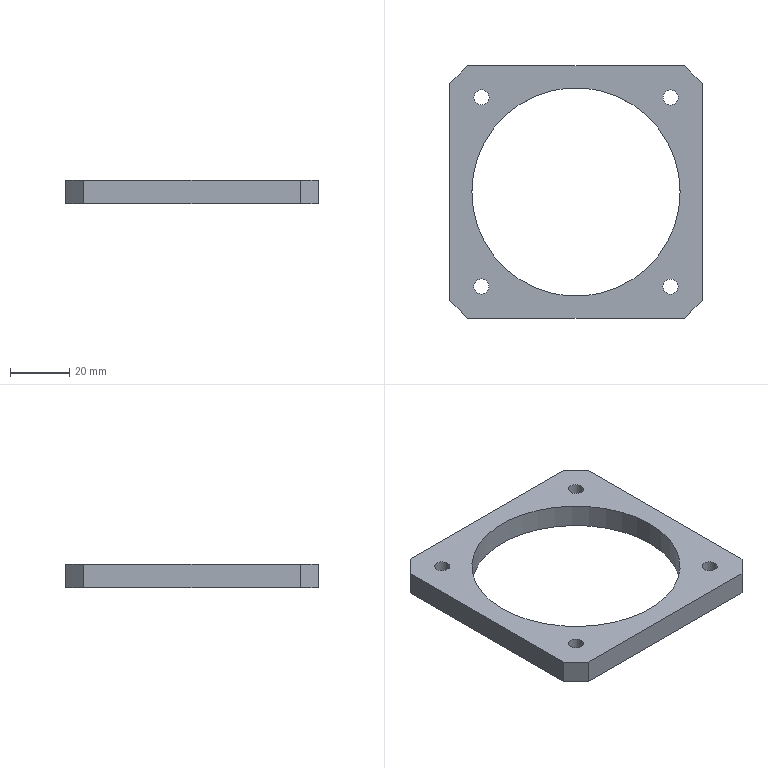NC program | NX | posted with a generic post | part box 85 x 85 x 8 mm
Lines 1 to 598 of 1875:
N10 G17 G21 G94 G90
(FACE_MILLING_COPY , TOOL : D63面刀)
N12 T08 M6
N14 G54
N16 G17 G0 G90 X105.5 Y-24.667 S3500 M3
N18 G43 Z20. H8
N20 Z3.05
N22 G94 G1 Z0.05 F1000.
N24 X74.
N26 X-74.
N28 X-105.5
N30 Z3.05
N32 G0 Z20.
N34 X105.5 Y24.667
N36 Z3.05
N38 G1 Z0.05
N40 X74.
N42 X-74.
N44 X-105.5
N46 Z3.05
N48 G0 Z20.
N50 M5
(DRILLING , TOOL : D8点钻)
N52 T07 M6
N54 G54
N56 G17 G0 G90 X0. Y0. S1200 M3
N58 G43 Z3. H7
N60 G94 G81 G99 Z-2. F250. R3.
N62 G80
N64 M5
(DRILLING_1 , TOOL : D8.3)
N66 T03 M6
N68 G54
N70 G17 G0 G90 X0. Y0. S1200 M3
N72 G43 Z3. H3
N74 G94 G81 G99 Z-12. F250. R3.
N76 G80
N78 M5
(FACE_MILLING , TOOL : D63面刀)
N80 T08 M6
N82 G54
N84 G17 G0 G90 X105.5 Y-24.667 S3500 M3
N86 G43 Z20. H8
N88 Z3.
N90 G94 G1 Z0. F800.
N92 X74.
N94 X-74.
N96 X-105.5
N98 Z3.
N100 G0 Z20.
N102 X105.5 Y24.667
N104 Z3.
N106 G1 Z0.
N108 X74.
N110 X-74.
N112 X-105.5
N114 Z3.
N116 G0 Z20.
N118 M5
(ADAPTIVE_MILLING , TOOL : D10C-25L-35L)
N120 T02 M6
N122 G54
N124 G17 G0 G90 X-53.678 Y0.03 S6500 M3
N126 G43 Z20. H2
N128 Z-6.
N130 G94 G1 Z-9. F2000.
N132 X-52.288 Y-0.463
N134 G3 X-51.05 Y0.03 R1.014
N136 X-50.503 Y2.195 R6.447
N138 X-50.235 Y8.306 R59.391
N140 G1 X-50.228 Y9.146
N142 X-50.222 Y10.166
N144 X-50.217 Y11.426
N146 X-50.213 Y13.046
N148 X-50.211 Y15.446
N150 X-50.209 Y19.946
N152 Y43.286
N154 X-50.208 Y43.346
N156 X-50.207 Y43.406
N158 X-50.206 Y43.466
N160 X-50.203 Y43.526
N162 X-50.199 Y43.586
N164 G2 X-48.102 Y47.433 R5.655
N166 X-43.686 Y49.49 R10.23
N168 X-38.026 Y50.093 R31.124
N170 X-26.147 Y50.189 R436.824
N172 G1 X-19.847 Y50.19
N174 X43.333 Y50.191
N176 X43.393 Y50.19
N178 X43.453 Y50.188
N180 X43.573 Y50.182
N182 X43.633 Y50.178
N184 G2 X47.505 Y48.006 R5.711
N186 X49.514 Y43.566 R10.377
N188 X50.104 Y37.724 R32.314
N190 X50.19 Y25.545 R519.78
N192 G1 Y17.625
N194 X50.191 Y-43.335
N196 X50.19 Y-43.395
N198 X50.188 Y-43.455
N200 X50.182 Y-43.575
N202 X50.178 Y-43.635
N204 G2 X48.005 Y-47.506 R5.712
N206 X43.506 Y-49.529 R10.425
N208 X37.722 Y-50.102 R33.162
N210 X26.503 Y-50.189 R472.894
N212 G1 X20.923 Y-50.19
N214 X-43.337 Y-50.191
N216 X-43.397 Y-50.19
N218 X-43.457 Y-50.188
N220 X-43.577 Y-50.182
N222 X-43.637 Y-50.178
N224 G2 X-47.469 Y-48.05 R5.701
N226 X-49.504 Y-43.622 R10.328
N228 X-50.103 Y-37.721 R32.321
N230 X-50.189 Y-26.501 R475.548
N232 G1 X-50.19 Y-20.861
N234 X-50.191 Y-3.341
N236 X-50.188 Y-3.161
N238 X-50.186 Y-3.041
N240 X-50.18 Y-2.861
N242 G2 X-49.726 Y2.097 R153.995
N244 G3 X-49.435 Y11.691 R130.242
N246 G1 X-49.43 Y12.831
N248 X-49.425 Y14.331
N250 X-49.422 Y16.371
N252 X-49.419 Y19.311
N254 X-49.418 Y25.311
N256 Y40.491
N258 G2 X-46.279 Y46.539 R7.433
N260 X-41.288 Y48.644 R12.586
N262 X-35.028 Y49.274 R36.96
N264 X-22.309 Y49.38 R464.734
N266 G1 X-16.549 Y49.381
N268 X40.571
N270 X40.691 Y49.38
N272 X40.811 Y49.377
N274 X40.931 Y49.372
N276 G2 X46.518 Y46.283 R7.42
N278 X48.64 Y41.299 R12.537
N280 X49.284 Y34.739 R38.062
N282 X49.38 Y20.94 R562.361
N284 G1 X49.381 Y12.18
N286 Y-40.56
N288 X49.38 Y-40.68
N290 X49.377 Y-40.8
N292 X49.372 Y-40.92
N294 G2 X46.292 Y-46.511 R7.42
N296 X41.427 Y-48.61 R12.43
N298 X35.051 Y-49.275 R35.605
N300 X22.152 Y-49.38 R477.842
N302 G1 X16.032 Y-49.381
N304 X-40.548
N306 X-40.668 Y-49.38
N308 X-40.788 Y-49.377
N310 X-40.908 Y-49.373
N312 X-40.968 Y-49.37
N314 G2 X-46.612 Y-46.159 R7.454
N316 X-48.658 Y-41.205 R12.716
N318 X-49.282 Y-34.763 R38.759
N320 X-49.381 Y-20.184 R586.068
N322 G1 Y-8.124
N324 Y-5.484
N326 X-49.379 Y-5.124
N328 X-49.375 Y-4.824
N330 X-49.368 Y-4.524
N332 G2 X-48.925 Y2.241 R213.822
N334 G3 X-48.637 Y15.256 R227.625
N336 G1 X-48.633 Y17.116
N338 X-48.63 Y19.636
N340 X-48.628 Y23.716
N342 X-48.627 Y35.416
N344 Y37.816
N346 X-48.625 Y38.176
N348 G2 X-44.355 Y45.949 R8.752
N350 X-38.853 Y47.916 R15.177
N352 X-31.743 Y48.488 R49.847
N354 X-16.743 Y48.572 R785.594
N356 G1 X-4.143
N358 X38.217
N360 X38.397 Y48.57
N362 X38.577 Y48.567
N364 X38.697 Y48.563
N366 X38.817 Y48.558
N368 G2 X45.848 Y44.487 R8.635
N370 X47.861 Y39.13 R14.769
N372 X48.477 Y32.144 R45.51
N374 X48.571 Y16.785 R691.053
N376 G1 X48.572 Y4.485
N378 Y-38.235
N380 X48.569 Y-38.475
N382 X48.565 Y-38.655
N384 X48.563 Y-38.715
N386 G2 X44.471 Y-45.857 R8.644
N388 X38.935 Y-47.9 R14.947
N390 X32.066 Y-48.48 R46.979
N392 X15.627 Y-48.572 R770.91
N394 G1 X-9.153
N396 X-38.193
N398 X-38.313 Y-48.571
N400 X-38.493 Y-48.569
N402 X-38.613 Y-48.566
N404 X-38.733 Y-48.562
N406 G2 X-45.867 Y-44.455 R8.647
N408 X-47.89 Y-38.975 R14.956
N410 X-48.49 Y-31.627 R49.124
N412 X-48.572 Y-15.967 R845.909
N414 X-48.537 Y-5.047 R550.163
N416 X-48.061 Y3.759 R992.687
N418 G3 X-47.841 Y19.897 R408.361
N420 G1 X-47.838 Y23.197
N422 X-47.837 Y29.317
N424 X-47.836 Y35.077
N426 X-47.833 Y35.617
N428 X-47.828 Y36.217
N430 X-47.824 Y36.457
N432 G2 X-46.48 Y41.68 R10.171
N434 X-41.618 Y45.808 R10.564
N436 X-39.71 Y46.527 R31.998
N438 X-38.421 Y47.273 R7.754
N440 X-36.474 Y47.65 R6.05
N442 G1 X-26.274
N444 X-26.034 Y47.66
N446 G2 X-14.395 Y47.761 R368.276
N448 G1 X-9.115 Y47.763
N450 X36.125
N452 X36.245 Y47.762
N454 X36.545 Y47.758
N456 X36.844 Y47.751
N458 G2 X45.139 Y42.88 R9.548
N460 X46.501 Y39.751 R15.537
N462 X47.273 Y38.421 R8.582
N464 X47.65 Y36.474 R6.05
N466 G1 Y26.274
N468 X47.66 Y26.034
N470 G2 X47.761 Y14.455 R366.235
N472 G1 X47.763 Y9.235
N474 Y-36.125
N476 X47.762 Y-36.245
N478 X47.758 Y-36.545
N480 X47.754 Y-36.724
N482 X47.75 Y-36.844
N484 G2 X42.879 Y-45.139 R9.551
N486 X39.75 Y-46.502 R15.425
N488 X38.421 Y-47.273 R8.784
N490 X36.474 Y-47.65 R6.05
N492 G1 X26.334
N494 X26.094 Y-47.66
N496 G2 X14.455 Y-47.761 R368.289
N498 G1 X9.175 Y-47.763
N500 X-36.125
N502 X-36.245 Y-47.762
N504 X-36.545 Y-47.758
N506 X-36.724 Y-47.754
N508 X-36.844 Y-47.75
N510 G2 X-45.045 Y-43.032 R9.521
N512 X-46.501 Y-39.749 R15.242
N514 X-47.273 Y-38.421 R8.325
N516 X-47.65 Y-36.474 R6.05
N518 G1 Y-26.274
N520 X-47.66 Y-26.034
N522 G2 X-47.761 Y-14.395 R368.277
N524 X-47.674 Y-4.437 R249.609
N526 G1 X-47.653 Y-3.957
N528 X-47.65 Y-3.895
N530 Y36.474
N532 X-47.647 Y36.526
N534 G2 X-46.777 Y39.368 R5.615
N536 X-42.111 Y44.175 R12.705
N538 G1 X-42.087 Y44.197
N540 X-40.16 Y46.123
N542 X-40.122 Y46.158
N544 X-39.565 Y46.615
N546 X-40.122 Y46.158
N548 X-40.16 Y46.123
N550 X-46.123 Y40.16
N552 X-46.158 Y40.122
N554 X-46.749 Y39.401
N556 X-46.806 Y39.316
N558 G2 X-48.524 Y40.337 R1.001
N560 G1 X-47.665 Y42.144 Z-8.9
N562 X-47.312 Y42.894
N564 X-46.948 Y43.638
N566 X-46.806 Y43.816
N568 X-41.5 Y49.122
N570 G2 X-39.403 Y50.273 R4.313
N572 X-36.943 Y50.593 R14.232
N574 G1 X-31.949 Y50.785
N576 X-29.456 Y50.832
N578 G2 X-28.604 Y50.38 R1.01
N580 G1 X-28.464 Y50.167
N582 X-27.368 Y48.494 Z-9.
N584 X-27.201 Y48.239
N586 X-27.025 Y47.989
N588 G3 X-26.274 Y47.65 R1.014
N590 G1 X36.474
N592 X36.526 Y47.647
N594 G2 X39.316 Y46.806 R5.544
N596 X44.136 Y42.151 R12.786
N598 G1 X44.161 Y42.123
N600 X46.123 Y40.16
N602 X46.158 Y40.122
N604 X46.615 Y39.565
N606 X46.158 Y40.122
N608 X46.123 Y40.16
N610 X40.16 Y46.123
N612 X40.122 Y46.158
N614 X39.401 Y46.749
N616 X39.316 Y46.806
N618 G2 X40.337 Y48.524 R1.001
N620 G1 X42.144 Y47.665 Z-8.9
N622 X42.894 Y47.312
N624 X43.638 Y46.948
N626 X43.816 Y46.806
N628 X49.122 Y41.5
N630 G2 X50.273 Y39.403 R4.313
N632 X50.593 Y36.943 R14.232
N634 G1 X50.785 Y31.949
N636 X50.832 Y29.456
N638 G2 X50.38 Y28.604 R1.01
N640 G1 X50.167 Y28.464
N642 X48.494 Y27.368 Z-9.
N644 X48.239 Y27.201
N646 X47.989 Y27.025
N648 G3 X47.65 Y26.274 R1.014
N650 G1 Y-36.474
N652 X47.647 Y-36.526
N654 G2 X46.806 Y-39.316 R5.544
N656 X42.151 Y-44.136 R12.777
N658 G1 X42.119 Y-44.164
N660 X40.16 Y-46.123
N662 X40.122 Y-46.158
N664 X39.565 Y-46.615
N666 X40.122 Y-46.158
N668 X40.16 Y-46.123
N670 X46.123 Y-40.16
N672 X46.158 Y-40.122
N674 X46.749 Y-39.401
N676 X46.806 Y-39.316
N678 G2 X48.524 Y-40.337 R1.001
N680 G1 X47.665 Y-42.144 Z-8.9
N682 X47.312 Y-42.894
N684 X46.948 Y-43.638
N686 X46.806 Y-43.816
N688 X41.5 Y-49.122
N690 G2 X39.403 Y-50.273 R4.311
N692 X36.943 Y-50.593 R14.261
N694 G1 X31.949 Y-50.785
N696 X29.516 Y-50.832
N698 G2 X28.664 Y-50.38 R1.01
N700 G1 X28.524 Y-50.167
N702 X27.428 Y-48.494 Z-9.
N704 X27.261 Y-48.238
N706 X27.085 Y-47.989
N708 G3 X26.334 Y-47.65 R1.014
N710 G1 X-36.474
N712 X-36.526 Y-47.647
N714 G2 X-39.316 Y-46.806 R5.544
N716 X-44.136 Y-42.151 R12.785
N718 G1 X-44.158 Y-42.125
N720 X-46.123 Y-40.16
N722 X-46.158 Y-40.122
N724 X-46.615 Y-39.565
N726 X-46.158 Y-40.122
N728 X-46.123 Y-40.16
N730 X-40.16 Y-46.123
N732 X-40.122 Y-46.158
N734 X-39.401 Y-46.749
N736 X-39.316 Y-46.806
N738 G2 X-40.337 Y-48.524 R1.001
N740 G1 X-42.144 Y-47.665 Z-8.9
N742 X-42.894 Y-47.312
N744 X-43.638 Y-46.948
N746 X-43.816 Y-46.806
N748 X-49.122 Y-41.5
N750 G2 X-50.273 Y-39.403 R4.313
N752 X-50.593 Y-36.943 R14.232
N754 G1 X-50.785 Y-31.949
N756 X-50.832 Y-29.456
N758 G2 X-50.38 Y-28.604 R1.01
N760 G1 X-50.07 Y-28.4
N762 X-48.397 Y-27.304 Z-9.
N764 X-48.19 Y-27.168
N766 X-47.989 Y-27.025
N768 G3 X-47.65 Y-26.274 R1.014
N770 G1 Y-3.894
N772 G3 X-48.503 Y-2.896 R1.014
N774 G1 X-50.09 Y-2.647
N776 Z-6.
N778 G0 Z20.
N780 M5
(PLANAR_MILL , TOOL : 8J-20L-30L)
N782 T03 M6
N784 G54
N786 G17 G0 G90 X-47.5 Y35.5 S3500 M3
N788 G43 Z20. H3
N790 Z-5.5
N792 G94 G1 Z-8.5 F800.
N794 G3 X-46.5 Y36.5 R1.
N796 G2 X-45.328 Y39.328 R4.
N798 G1 X-39.328 Y45.328
N800 G2 X-36.5 Y46.5 R4.
N802 G1 X36.5
N804 G2 X39.328 Y45.328 R4.
N806 G1 X45.328 Y39.328
N808 G2 X46.5 Y36.5 R4.
N810 G1 Y-36.5
N812 G2 X45.328 Y-39.328 R4.
N814 G1 X39.328 Y-45.328
N816 G2 X36.5 Y-46.5 R4.
N818 G1 X-36.5
N820 G2 X-39.328 Y-45.328 R4.
N822 G1 X-45.328 Y-39.328
N824 G2 X-46.5 Y-36.5 R4.
N826 G1 Y36.5
N828 G3 X-47.5 Y37.5 R1.
N830 G1 Z-5.5
N832 G0 Z20.
N834 M5
(DRILLING_2 , TOOL : D8点钻)
N836 T07 M6
N838 G54
N840 G17 G0 G90 X-31.82 Y31.82 S1200 M3
N842 G43 Z20. H7
N844 G94 G81 G99 Z-3. F200. R3.
N846 X31.82
N848 Y-31.82
N850 X-31.82
N852 G80
N854 G0 X-31.82 Y-31.82 Z20.
N856 M5
(DRILLING_2_COPY , TOOL : D5钻头)
N858 T04 M6
N860 G54
N862 G17 G0 G90 X-31.82 Y31.82 S1200 M3
N864 G43 Z20. H4
N866 G94 G81 G99 Z-13. F200. R3.
N868 X31.82
N870 Y-31.82
N872 X-31.82
N874 G80
N876 G0 X-31.82 Y-31.82 Z20.
N878 M5
(PLANAR_MILL_1 , TOOL : D50面刀)
N880 T11 M6
N882 G54
N884 G17 G0 G90 X-64.05 Y-7. S3500 M3
N886 G43 Z20. H11
N888 Z3.05
N890 G94 G1 Z0.05 F800.
N892 G3 X-57.05 Y0. R7.
N894 G2 X0. Y57.05 R57.05
N896 X-57.05 Y0. R-57.05
N898 G3 X-64.05 Y7. R7.
N900 G1 Z3.05
N902 G0 Z20.
N904 M5
(PLANAR_MILL_1_COPY , TOOL : D63面刀)
N906 T08 M6
N908 G54
N910 G17 G0 G90 X-70.55 Y-7. S3500 M3
N912 G43 Z20. H8
N914 Z3.
N916 G94 G1 Z0. F800.
N918 G3 X-63.55 Y0. R7.
N920 G2 X0. Y63.55 R63.55
N922 X-63.55 Y0. R-63.55
N924 G3 X-70.55 Y7. R7.
N926 G1 Z3.
N928 G0 Z20.
N930 M5
(PLANAR_MILL_2 , TOOL : D4反刮刀)
N932 T06 M6
N934 G54
N936 G17 G0 G90 X-46. Y-2. S3500 M3
N938 G43 Z20. H6
N940 Z2.5
N942 G94 G1 Z-0.5 F1000.
N944 G3 X-44. Y0. R2.
N946 G1 Y36.5
N948 G2 X-43.561 Y37.561 R1.5
N950 G1 X-37.561 Y43.561
N952 G2 X-36.5 Y44. R1.5
N954 G1 X36.5
N956 G2 X37.561 Y43.561 R1.5
N958 G1 X43.561 Y37.561
N960 G2 X44. Y36.5 R1.5
N962 G1 Y-36.5
N964 G2 X43.561 Y-37.561 R1.5
N966 G1 X37.561 Y-43.561
N968 G2 X36.5 Y-44. R1.5
N970 G1 X-36.5
N972 G2 X-37.561 Y-43.561 R1.5
N974 G1 X-43.561 Y-37.561
N976 G2 X-44. Y-36.5 R1.5
N978 G1 Y0.
N980 G3 X-46. Y2. R2.
N982 G1 Z2.5
N984 G0 Z20.
(PLANAR_MILL_2_COPY , TOOL : D4反刮刀)
N986 X-46.35 Y-2.
N988 Z-5.85
N990 G1 Z-8.85
N992 G3 X-44.35 Y0. R2.
N994 G1 Y36.5
N996 G2 X-43.808 Y37.808 R1.85
N998 G1 X-37.808 Y43.808
N1000 G2 X-36.5 Y44.35 R1.85
N1002 G1 X36.5
N1004 G2 X37.808 Y43.808 R1.85
N1006 G1 X43.808 Y37.808
N1008 G2 X44.35 Y36.5 R1.85
N1010 G1 Y-36.5
N1012 G2 X43.808 Y-37.808 R1.85
N1014 G1 X37.808 Y-43.808
N1016 G2 X36.5 Y-44.35 R1.85
N1018 G1 X-36.5
N1020 G2 X-37.808 Y-43.808 R1.85
N1022 G1 X-43.808 Y-37.808
N1024 G2 X-44.35 Y-36.5 R1.85
N1026 G1 Y0.
N1028 G3 X-46.35 Y2. R2.
N1030 G1 Z-5.85
N1032 G0 Z20.
(PLANAR_MILL_4 , TOOL : D4反刮刀)
N1034 X-31.83 Y-31.72
N1036 Z-7.
N1038 G1 Z-9. F800.
N1040 X-31.92 Y-30.82
N1042 G3 X-32.92 Y-31.82 R1.
N1044 X-31.82 Y-32.92 R1.1
N1046 X-32.92 Y-31.82 R-1.1
N1048 X-31.92 Y-32.82 R1.
N1050 G1 X-31.83 Y-31.919
N1052 Z-7.
N1054 G0 Z20.
N1056 X31.81 Y-31.72
N1058 Z-7.
N1060 G1 Z-9.
N1062 X31.72 Y-30.82
N1064 G3 X30.72 Y-31.82 R1.
N1066 X31.82 Y-32.92 R1.1
N1068 X30.72 Y-31.82 R-1.1
N1070 X31.72 Y-32.82 R1.
N1072 G1 X31.81 Y-31.919
N1074 Z-7.
N1076 G0 Z20.
N1078 Y31.919
N1080 Z-7.
N1082 G1 Z-9.
N1084 X31.72 Y32.82
N1086 G3 X30.72 Y31.82 R1.
N1088 X31.82 Y30.72 R1.1
N1090 X30.72 Y31.82 R-1.1
N1092 X31.72 Y30.82 R1.
N1094 G1 X31.81 Y31.72
N1096 Z-7.
N1098 G0 Z20.
N1100 X-31.83 Y31.919
N1102 Z-7.
N1104 G1 Z-9.
N1106 X-31.92 Y32.82
N1108 G3 X-32.92 Y31.82 R1.
N1110 X-31.82 Y30.72 R1.1
N1112 X-32.92 Y31.82 R-1.1
N1114 X-31.92 Y30.82 R1.
N1116 G1 X-31.83 Y31.72
N1118 Z-7.
N1120 G0 Z20.
N1122 M5